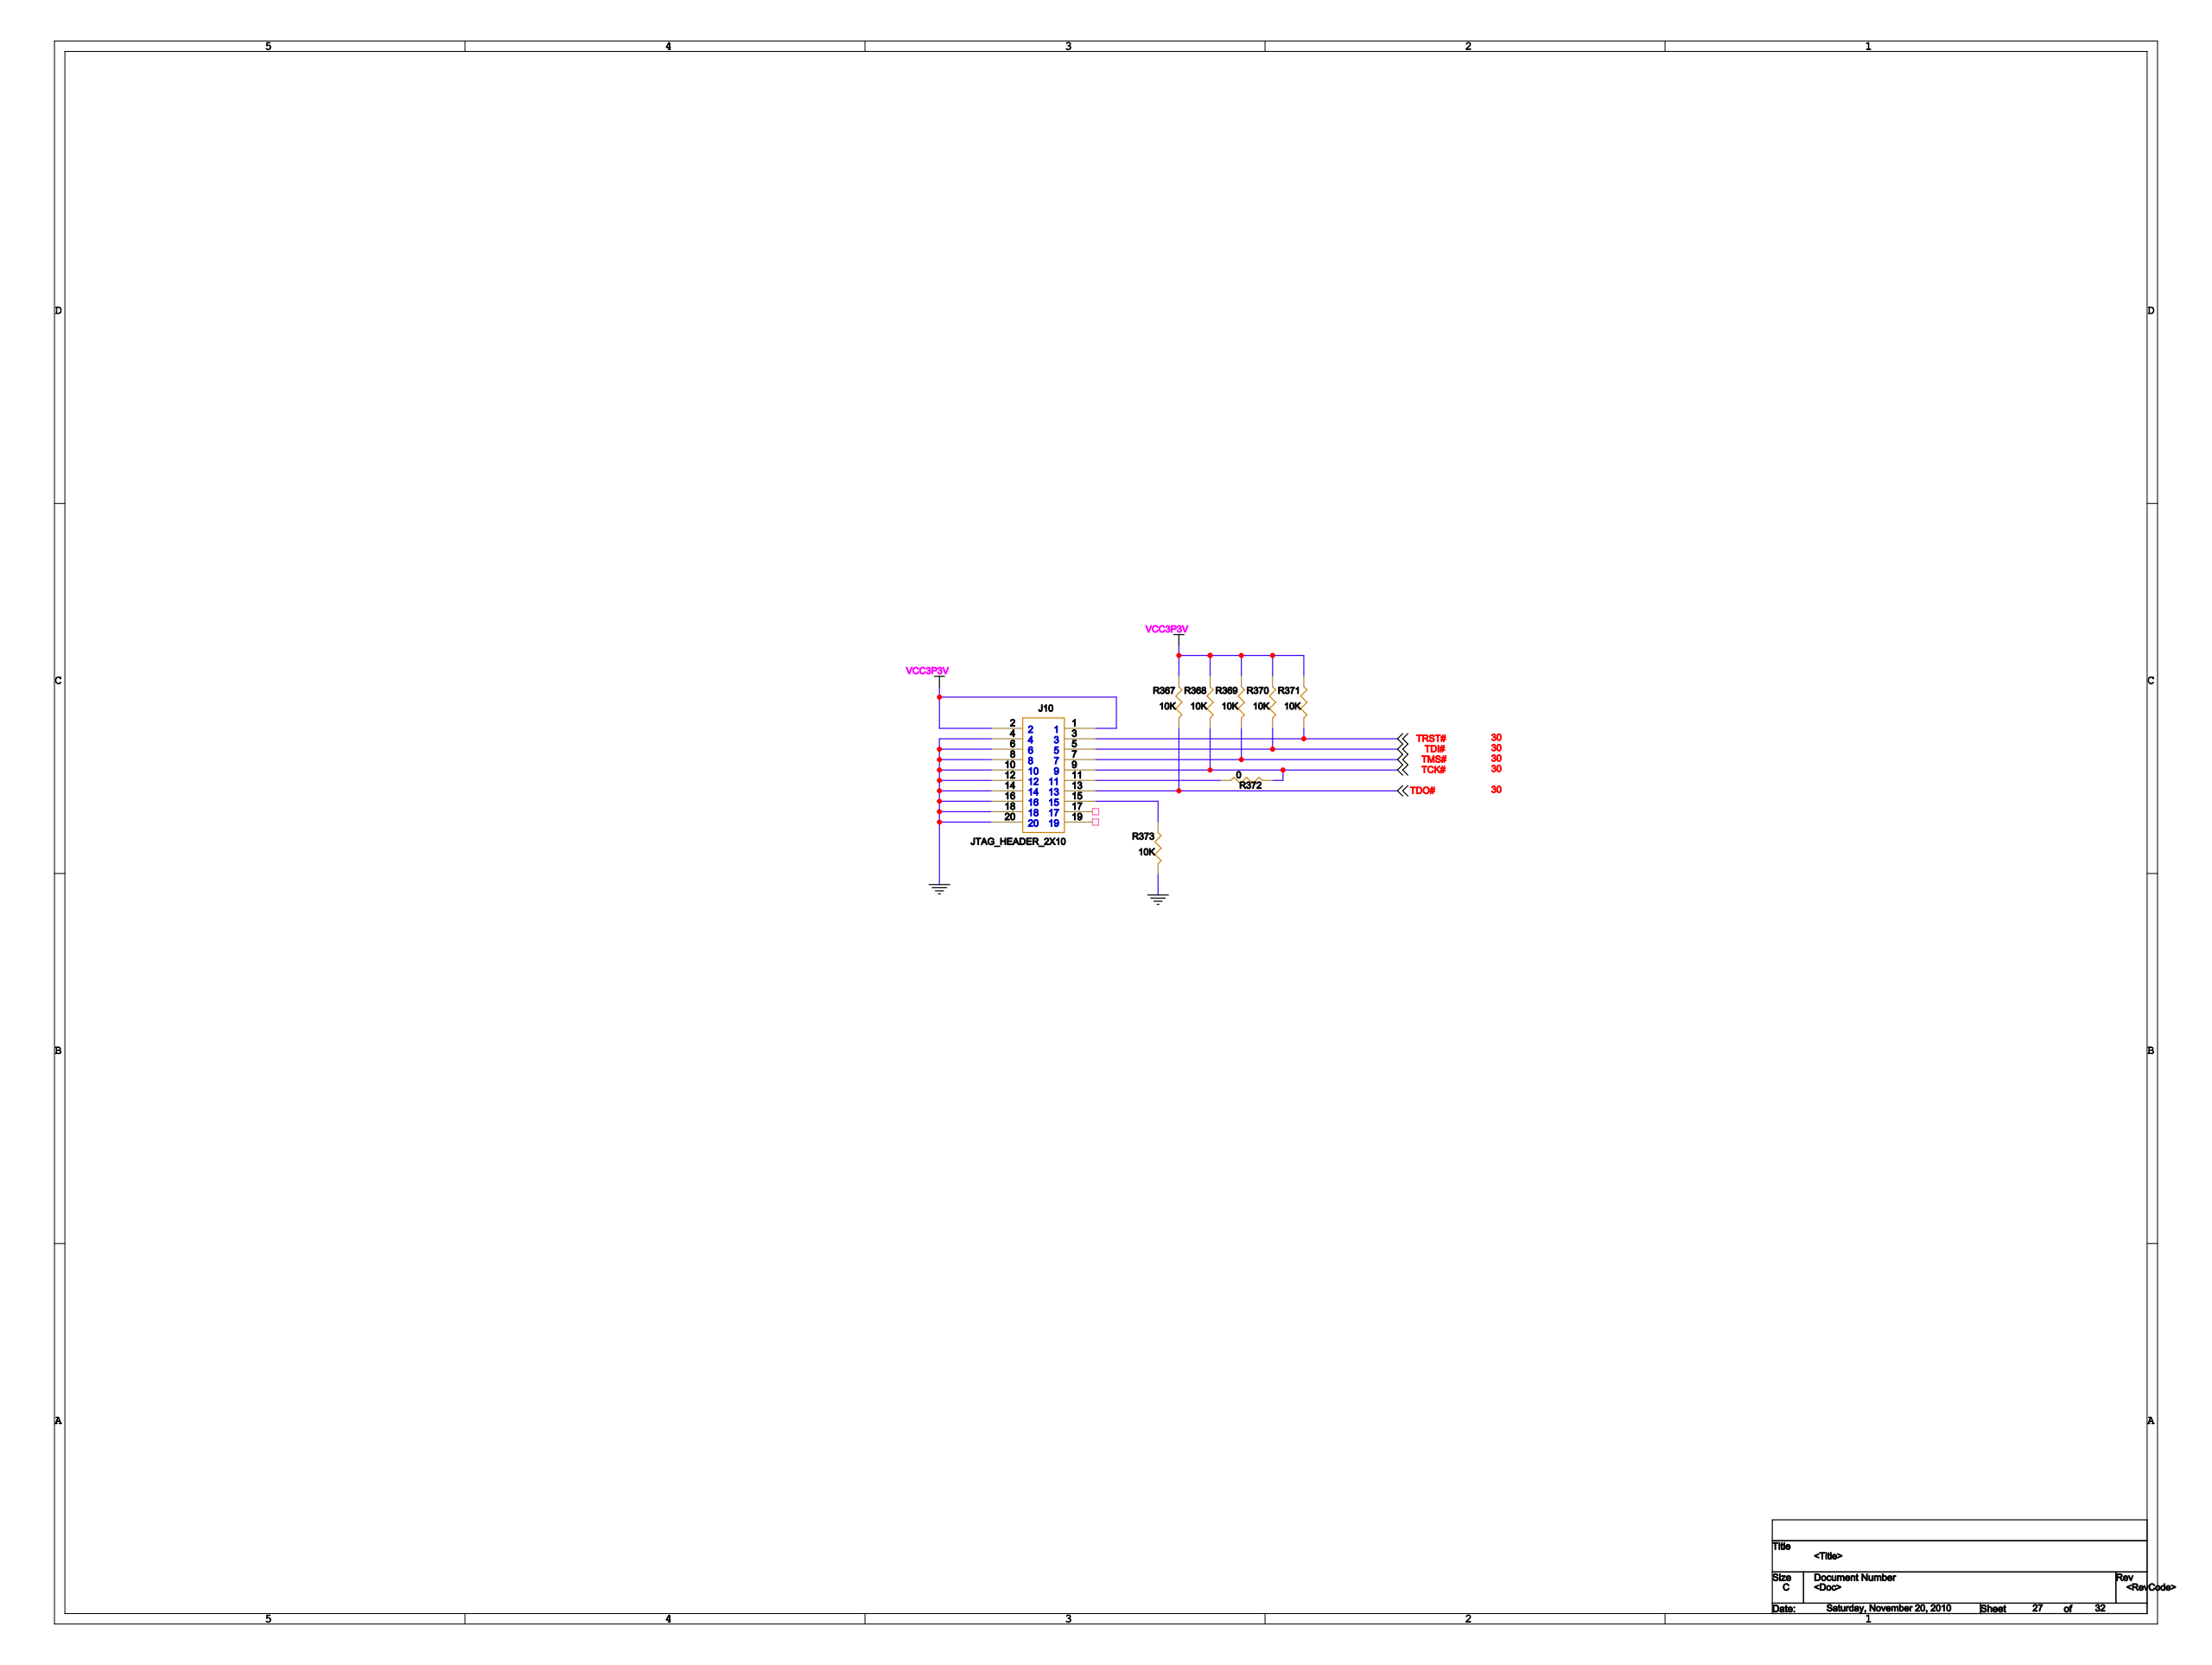Circuit board | Cadence Allegro | 1001 parts | 1318 nets | one sheet of the schematic
Parts on this sheet (reference | value | footprint):
J10 | JTAG_HEADER_2X10 | JTAG_HEADER_2X10
R367 | 10K | 0603
R368 | 10K | 0603
R369 | 10K | 0603
R370 | 10K | 0603
R371 | 10K | 0603
R372 | 0 | 0603
R373 | 10K | 0603
Nets of these parts (net: part-pin ...):
GND: J10-4 J10-6 J10-8 J10-10 J10-12 J10-14 J10-16 J10-18 J10-20 R373-1
TRST#: J10-3 R371-1
TCK#: J10-9 R368-1 R372-1
TDO#: J10-13 R367-1
TDI#: J10-5 R370-1
TMS#: J10-7 R369-1
VCC3P3V: J10-1 J10-2 R367-2 R368-2 R369-2 R370-2 R371-2
N16976419: J10-11 R372-2
N16975550: J10-15 R373-2